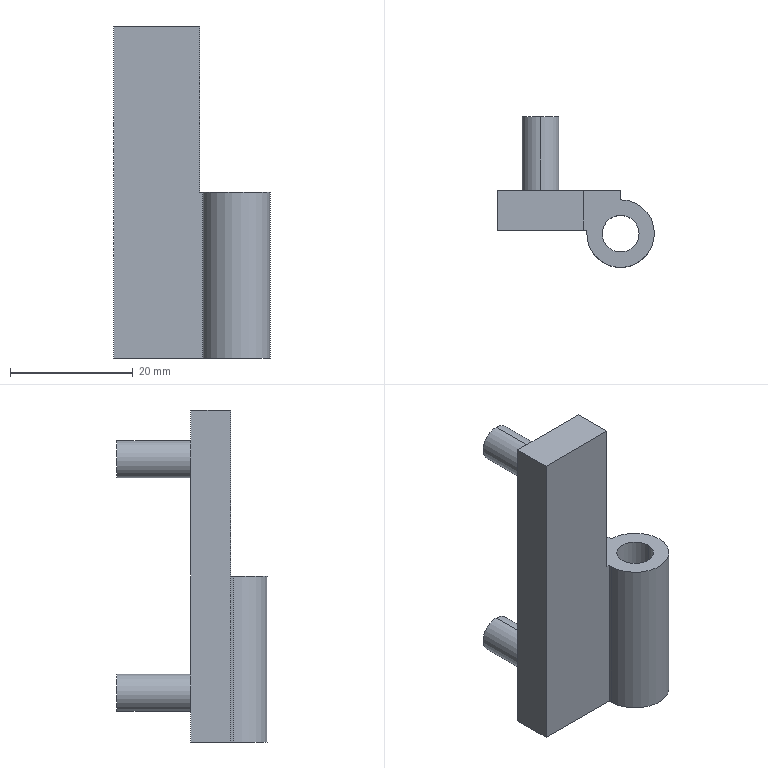Part | STEP file | Hinge leaf | 1 solid | 19 faces | box 25.5 x 24.5 x 54 mm | volume 7881 mm3 | plane 10 | cylinder 9 | commonest cylinder face diameters 6 x6 11 x3
STEP:
#1=CARTESIAN_POINT('',(0.,0.,0.));
#2=DIRECTION('',(0.,0.,1.));
#3=DIRECTION('',(1.,0.,0.));
#4=AXIS2_PLACEMENT_3D('',#1,#2,#3);
#5=CARTESIAN_POINT('',(7.,12.,43.));
#6=VERTEX_POINT('',#5);
#7=CARTESIAN_POINT('',(7.,12.,49.));
#8=VERTEX_POINT('',#7);
#9=CARTESIAN_POINT('',(7.,12.,46.));
#10=DIRECTION('',(0.,-1.,0.));
#11=DIRECTION('',(0.,0.,-1.));
#12=AXIS2_PLACEMENT_3D('',#9,#10,#11);
#13=CIRCLE('',#12,3.);
#14=CARTESIAN_POINT('',(7.,12.,46.));
#15=DIRECTION('',(0.,-1.,0.));
#16=DIRECTION('',(0.,0.,-1.));
#17=AXIS2_PLACEMENT_3D('',#14,#15,#16);
#18=CYLINDRICAL_SURFACE('',#17,3.);
#19=CARTESIAN_POINT('',(0.,0.));
#20=DIRECTION('',(1.,0.));
#21=VECTOR('',#20,1.);
#22=LINE('',#19,#21);
#23=(GEOMETRIC_REPRESENTATION_CONTEXT(2)PARAMETRIC_REPRESENTATION_CONTEXT()REPRESENTATION_CONTEXT('',''));
#24=DEFINITIONAL_REPRESENTATION('',(#22),#23);
#25=PCURVE('',#18,#24);
#26=CARTESIAN_POINT('',(7.,12.,46.));
#27=DIRECTION('',(0.,1.,0.));
#28=DIRECTION('',(0.,0.,1.));
#29=AXIS2_PLACEMENT_3D('',#26,#27,#28);
#30=PLANE('',#29);
#31=CARTESIAN_POINT('',(-3.,0.));
#32=CARTESIAN_POINT('',(-3.,5.196));
#33=CARTESIAN_POINT('',(1.5,2.598));
#34=CARTESIAN_POINT('',(6.,0.));
#35=CARTESIAN_POINT('',(1.5,-2.598));
#36=CARTESIAN_POINT('',(-3.,-5.196));
#37=CARTESIAN_POINT('',(-3.,0.));
#38=(BOUNDED_CURVE()B_SPLINE_CURVE(2,(#31,#32,#33,#34,#35,#36,#37),.UNSPECIFIED.,.T.,.F.)B_SPLINE_CURVE_WITH_KNOTS((1,2,2,2,2,1),(-2.094,0.,2.094,4.189,6.283,8.378),.UNSPECIFIED.)CURVE()GEOMETRIC_REPRESENTATION_ITEM()RATIONAL_B_SPLINE_CURVE((1.,0.5,1.,0.5,1.,0.5,1.))REPRESENTATION_ITEM(''));
#39=(GEOMETRIC_REPRESENTATION_CONTEXT(2)PARAMETRIC_REPRESENTATION_CONTEXT()REPRESENTATION_CONTEXT('',''));
#40=DEFINITIONAL_REPRESENTATION('',(#38),#39);
#41=PCURVE('',#30,#40);
#42=SURFACE_CURVE('',#13,(#25,#41),.PCURVE_S1.);
#43=EDGE_CURVE('',#6,#8,#42,.T.);
#44=ORIENTED_EDGE('',*,*,#43,.T.);
#45=CARTESIAN_POINT('',(7.,0.,49.));
#46=VERTEX_POINT('',#45);
#47=CARTESIAN_POINT('',(7.,12.,49.));
#48=DIRECTION('',(0.,-1.,0.));
#49=VECTOR('',#48,1.);
#50=LINE('',#47,#49);
#51=CARTESIAN_POINT('',(3.142,0.));
#52=DIRECTION('',(0.,1.));
#53=VECTOR('',#52,1.);
#54=LINE('',#51,#53);
#55=(GEOMETRIC_REPRESENTATION_CONTEXT(2)PARAMETRIC_REPRESENTATION_CONTEXT()REPRESENTATION_CONTEXT('',''));
#56=DEFINITIONAL_REPRESENTATION('',(#54),#55);
#57=PCURVE('',#18,#56);
#58=CARTESIAN_POINT('',(7.,12.,46.));
#59=DIRECTION('',(0.,-1.,0.));
#60=DIRECTION('',(0.,0.,-1.));
#61=AXIS2_PLACEMENT_3D('',#58,#59,#60);
#62=CYLINDRICAL_SURFACE('',#61,3.);
#63=CARTESIAN_POINT('',(3.142,0.));
#64=DIRECTION('',(0.,1.));
#65=VECTOR('',#64,1.);
#66=LINE('',#63,#65);
#67=(GEOMETRIC_REPRESENTATION_CONTEXT(2)PARAMETRIC_REPRESENTATION_CONTEXT()REPRESENTATION_CONTEXT('',''));
#68=DEFINITIONAL_REPRESENTATION('',(#66),#67);
#69=PCURVE('',#62,#68);
#70=SURFACE_CURVE('',#50,(#57,#69),.PCURVE_S1.);
#71=EDGE_CURVE('',#8,#46,#70,.T.);
#72=ORIENTED_EDGE('',*,*,#71,.T.);
#73=CARTESIAN_POINT('',(7.,0.,43.));
#74=VERTEX_POINT('',#73);
#75=CARTESIAN_POINT('',(7.,0.,46.));
#76=DIRECTION('',(0.,1.,0.));
#77=DIRECTION('',(0.,0.,-1.));
#78=AXIS2_PLACEMENT_3D('',#75,#76,#77);
#79=CIRCLE('',#78,3.);
#80=CARTESIAN_POINT('',(6.283,12.));
#81=DIRECTION('',(-1.,0.));
#82=VECTOR('',#81,1.);
#83=LINE('',#80,#82);
#84=(GEOMETRIC_REPRESENTATION_CONTEXT(2)PARAMETRIC_REPRESENTATION_CONTEXT()REPRESENTATION_CONTEXT('',''));
#85=DEFINITIONAL_REPRESENTATION('',(#83),#84);
#86=PCURVE('',#18,#85);
#87=CARTESIAN_POINT('',(0.,0.,54.));
#88=DIRECTION('',(0.,-1.,0.));
#89=DIRECTION('',(0.,0.,-1.));
#90=AXIS2_PLACEMENT_3D('',#87,#88,#89);
#91=PLANE('',#90);
#92=CARTESIAN_POINT('',(11.,7.));
#93=CARTESIAN_POINT('',(11.,1.804));
#94=CARTESIAN_POINT('',(6.5,4.402));
#95=CARTESIAN_POINT('',(2.,7.));
#96=CARTESIAN_POINT('',(6.5,9.598));
#97=CARTESIAN_POINT('',(11.,12.196));
#98=CARTESIAN_POINT('',(11.,7.));
#99=(BOUNDED_CURVE()B_SPLINE_CURVE(2,(#92,#93,#94,#95,#96,#97,#98),.UNSPECIFIED.,.T.,.F.)B_SPLINE_CURVE_WITH_KNOTS((1,2,2,2,2,1),(-2.094,0.,2.094,4.189,6.283,8.378),.UNSPECIFIED.)CURVE()GEOMETRIC_REPRESENTATION_ITEM()RATIONAL_B_SPLINE_CURVE((1.,0.5,1.,0.5,1.,0.5,1.))REPRESENTATION_ITEM(''));
#100=(GEOMETRIC_REPRESENTATION_CONTEXT(2)PARAMETRIC_REPRESENTATION_CONTEXT()REPRESENTATION_CONTEXT('',''));
#101=DEFINITIONAL_REPRESENTATION('',(#99),#100);
#102=PCURVE('',#91,#101);
#103=SURFACE_CURVE('',#79,(#86,#102),.PCURVE_S1.);
#104=EDGE_CURVE('',#46,#74,#103,.T.);
#105=ORIENTED_EDGE('',*,*,#104,.T.);
#106=CARTESIAN_POINT('',(7.,12.,43.));
#107=DIRECTION('',(0.,-1.,0.));
#108=VECTOR('',#107,1.);
#109=LINE('',#106,#108);
#110=CARTESIAN_POINT('',(0.,0.));
#111=DIRECTION('',(0.,1.));
#112=VECTOR('',#111,1.);
#113=LINE('',#110,#112);
#114=(GEOMETRIC_REPRESENTATION_CONTEXT(2)PARAMETRIC_REPRESENTATION_CONTEXT()REPRESENTATION_CONTEXT('',''));
#115=DEFINITIONAL_REPRESENTATION('',(#113),#114);
#116=PCURVE('',#18,#115);
#117=CARTESIAN_POINT('',(6.283,0.));
#118=DIRECTION('',(0.,1.));
#119=VECTOR('',#118,1.);
#120=LINE('',#117,#119);
#121=(GEOMETRIC_REPRESENTATION_CONTEXT(2)PARAMETRIC_REPRESENTATION_CONTEXT()REPRESENTATION_CONTEXT('',''));
#122=DEFINITIONAL_REPRESENTATION('',(#120),#121);
#123=PCURVE('',#62,#122);
#124=SURFACE_CURVE('',#109,(#116,#123),.PCURVE_S1.);
#125=EDGE_CURVE('',#6,#74,#124,.T.);
#126=ORIENTED_EDGE('',*,*,#125,.F.);
#127=EDGE_LOOP('',(#44,#72,#105,#126));
#128=FACE_BOUND('',#127,.T.);
#129=ADVANCED_FACE('',(#128),#18,.T.);
#130=CARTESIAN_POINT('',(7.,12.,5.));
#131=VERTEX_POINT('',#130);
#132=CARTESIAN_POINT('',(7.,12.,11.));
#133=VERTEX_POINT('',#132);
#134=CARTESIAN_POINT('',(7.,12.,8.));
#135=DIRECTION('',(0.,-1.,0.));
#136=DIRECTION('',(0.,0.,-1.));
#137=AXIS2_PLACEMENT_3D('',#134,#135,#136);
#138=CIRCLE('',#137,3.);
#139=CARTESIAN_POINT('',(7.,12.,8.));
#140=DIRECTION('',(0.,-1.,0.));
#141=DIRECTION('',(0.,0.,-1.));
#142=AXIS2_PLACEMENT_3D('',#139,#140,#141);
#143=CYLINDRICAL_SURFACE('',#142,3.);
#144=CARTESIAN_POINT('',(0.,0.));
#145=DIRECTION('',(1.,0.));
#146=VECTOR('',#145,1.);
#147=LINE('',#144,#146);
#148=(GEOMETRIC_REPRESENTATION_CONTEXT(2)PARAMETRIC_REPRESENTATION_CONTEXT()REPRESENTATION_CONTEXT('',''));
#149=DEFINITIONAL_REPRESENTATION('',(#147),#148);
#150=PCURVE('',#143,#149);
#151=CARTESIAN_POINT('',(7.,12.,8.));
#152=DIRECTION('',(0.,1.,0.));
#153=DIRECTION('',(0.,0.,1.));
#154=AXIS2_PLACEMENT_3D('',#151,#152,#153);
#155=PLANE('',#154);
#156=CARTESIAN_POINT('',(-3.,0.));
#157=CARTESIAN_POINT('',(-3.,5.196));
#158=CARTESIAN_POINT('',(1.5,2.598));
#159=CARTESIAN_POINT('',(6.,0.));
#160=CARTESIAN_POINT('',(1.5,-2.598));
#161=CARTESIAN_POINT('',(-3.,-5.196));
#162=CARTESIAN_POINT('',(-3.,0.));
#163=(BOUNDED_CURVE()B_SPLINE_CURVE(2,(#156,#157,#158,#159,#160,#161,#162),.UNSPECIFIED.,.T.,.F.)B_SPLINE_CURVE_WITH_KNOTS((1,2,2,2,2,1),(-2.094,0.,2.094,4.189,6.283,8.378),.UNSPECIFIED.)CURVE()GEOMETRIC_REPRESENTATION_ITEM()RATIONAL_B_SPLINE_CURVE((1.,0.5,1.,0.5,1.,0.5,1.))REPRESENTATION_ITEM(''));
#164=(GEOMETRIC_REPRESENTATION_CONTEXT(2)PARAMETRIC_REPRESENTATION_CONTEXT()REPRESENTATION_CONTEXT('',''));
#165=DEFINITIONAL_REPRESENTATION('',(#163),#164);
#166=PCURVE('',#155,#165);
#167=SURFACE_CURVE('',#138,(#150,#166),.PCURVE_S1.);
#168=EDGE_CURVE('',#131,#133,#167,.T.);
#169=ORIENTED_EDGE('',*,*,#168,.T.);
#170=CARTESIAN_POINT('',(7.,0.,11.));
#171=VERTEX_POINT('',#170);
#172=CARTESIAN_POINT('',(7.,12.,11.));
#173=DIRECTION('',(0.,-1.,0.));
#174=VECTOR('',#173,1.);
#175=LINE('',#172,#174);
#176=CARTESIAN_POINT('',(3.142,0.));
#177=DIRECTION('',(0.,1.));
#178=VECTOR('',#177,1.);
#179=LINE('',#176,#178);
#180=(GEOMETRIC_REPRESENTATION_CONTEXT(2)PARAMETRIC_REPRESENTATION_CONTEXT()REPRESENTATION_CONTEXT('',''));
#181=DEFINITIONAL_REPRESENTATION('',(#179),#180);
#182=PCURVE('',#143,#181);
#183=CARTESIAN_POINT('',(7.,12.,8.));
#184=DIRECTION('',(0.,-1.,0.));
#185=DIRECTION('',(0.,0.,-1.));
#186=AXIS2_PLACEMENT_3D('',#183,#184,#185);
#187=CYLINDRICAL_SURFACE('',#186,3.);
#188=CARTESIAN_POINT('',(3.142,0.));
#189=DIRECTION('',(0.,1.));
#190=VECTOR('',#189,1.);
#191=LINE('',#188,#190);
#192=(GEOMETRIC_REPRESENTATION_CONTEXT(2)PARAMETRIC_REPRESENTATION_CONTEXT()REPRESENTATION_CONTEXT('',''));
#193=DEFINITIONAL_REPRESENTATION('',(#191),#192);
#194=PCURVE('',#187,#193);
#195=SURFACE_CURVE('',#175,(#182,#194),.PCURVE_S1.);
#196=EDGE_CURVE('',#133,#171,#195,.T.);
#197=ORIENTED_EDGE('',*,*,#196,.T.);
#198=CARTESIAN_POINT('',(7.,0.,5.));
#199=VERTEX_POINT('',#198);
#200=CARTESIAN_POINT('',(7.,0.,8.));
#201=DIRECTION('',(0.,1.,0.));
#202=DIRECTION('',(0.,0.,-1.));
#203=AXIS2_PLACEMENT_3D('',#200,#201,#202);
#204=CIRCLE('',#203,3.);
#205=CARTESIAN_POINT('',(6.283,12.));
#206=DIRECTION('',(-1.,0.));
#207=VECTOR('',#206,1.);
#208=LINE('',#205,#207);
#209=(GEOMETRIC_REPRESENTATION_CONTEXT(2)PARAMETRIC_REPRESENTATION_CONTEXT()REPRESENTATION_CONTEXT('',''));
#210=DEFINITIONAL_REPRESENTATION('',(#208),#209);
#211=PCURVE('',#143,#210);
#212=CARTESIAN_POINT('',(49.,7.));
#213=CARTESIAN_POINT('',(49.,1.804));
#214=CARTESIAN_POINT('',(44.5,4.402));
#215=CARTESIAN_POINT('',(40.,7.));
#216=CARTESIAN_POINT('',(44.5,9.598));
#217=CARTESIAN_POINT('',(49.,12.196));
#218=CARTESIAN_POINT('',(49.,7.));
#219=(BOUNDED_CURVE()B_SPLINE_CURVE(2,(#212,#213,#214,#215,#216,#217,#218),.UNSPECIFIED.,.T.,.F.)B_SPLINE_CURVE_WITH_KNOTS((1,2,2,2,2,1),(-2.094,0.,2.094,4.189,6.283,8.378),.UNSPECIFIED.)CURVE()GEOMETRIC_REPRESENTATION_ITEM()RATIONAL_B_SPLINE_CURVE((1.,0.5,1.,0.5,1.,0.5,1.))REPRESENTATION_ITEM(''));
#220=(GEOMETRIC_REPRESENTATION_CONTEXT(2)PARAMETRIC_REPRESENTATION_CONTEXT()REPRESENTATION_CONTEXT('',''));
#221=DEFINITIONAL_REPRESENTATION('',(#219),#220);
#222=PCURVE('',#91,#221);
#223=SURFACE_CURVE('',#204,(#211,#222),.PCURVE_S1.);
#224=EDGE_CURVE('',#171,#199,#223,.T.);
#225=ORIENTED_EDGE('',*,*,#224,.T.);
#226=CARTESIAN_POINT('',(7.,12.,5.));
#227=DIRECTION('',(0.,-1.,0.));
#228=VECTOR('',#227,1.);
#229=LINE('',#226,#228);
#230=CARTESIAN_POINT('',(0.,0.));
#231=DIRECTION('',(0.,1.));
#232=VECTOR('',#231,1.);
#233=LINE('',#230,#232);
#234=(GEOMETRIC_REPRESENTATION_CONTEXT(2)PARAMETRIC_REPRESENTATION_CONTEXT()REPRESENTATION_CONTEXT('',''));
#235=DEFINITIONAL_REPRESENTATION('',(#233),#234);
#236=PCURVE('',#143,#235);
#237=CARTESIAN_POINT('',(6.283,0.));
#238=DIRECTION('',(0.,1.));
#239=VECTOR('',#238,1.);
#240=LINE('',#237,#239);
#241=(GEOMETRIC_REPRESENTATION_CONTEXT(2)PARAMETRIC_REPRESENTATION_CONTEXT()REPRESENTATION_CONTEXT('',''));
#242=DEFINITIONAL_REPRESENTATION('',(#240),#241);
#243=PCURVE('',#187,#242);
#244=SURFACE_CURVE('',#229,(#236,#243),.PCURVE_S1.);
#245=EDGE_CURVE('',#131,#199,#244,.T.);
#246=ORIENTED_EDGE('',*,*,#245,.F.);
#247=EDGE_LOOP('',(#169,#197,#225,#246));
#248=FACE_BOUND('',#247,.T.);
#249=ADVANCED_FACE('',(#248),#143,.T.);
#250=CARTESIAN_POINT('',(25.5,-7.,27.));
#251=VERTEX_POINT('',#250);
#252=CARTESIAN_POINT('',(20.,-1.5,27.));
#253=VERTEX_POINT('',#252);
#254=CARTESIAN_POINT('',(20.,-7.,27.));
#255=DIRECTION('',(0.,0.,1.));
#256=DIRECTION('',(-1.,0.,0.));
#257=AXIS2_PLACEMENT_3D('',#254,#255,#256);
#258=CIRCLE('',#257,5.5);
#259=CARTESIAN_POINT('',(20.,-7.,54.));
#260=DIRECTION('',(0.,0.,-1.));
#261=DIRECTION('',(-1.,0.,0.));
#262=AXIS2_PLACEMENT_3D('',#259,#260,#261);
#263=CYLINDRICAL_SURFACE('',#262,5.5);
#264=CARTESIAN_POINT('',(6.283,27.));
#265=DIRECTION('',(-1.,0.));
#266=VECTOR('',#265,1.);
#267=LINE('',#264,#266);
#268=(GEOMETRIC_REPRESENTATION_CONTEXT(2)PARAMETRIC_REPRESENTATION_CONTEXT()REPRESENTATION_CONTEXT('',''));
#269=DEFINITIONAL_REPRESENTATION('',(#267),#268);
#270=PCURVE('',#263,#269);
#271=CARTESIAN_POINT('',(14.,-14.282,27.));
#272=DIRECTION('',(0.,0.,1.));
#273=DIRECTION('',(1.,0.,0.));
#274=AXIS2_PLACEMENT_3D('',#271,#272,#273);
#275=PLANE('',#274);
#276=CARTESIAN_POINT('',(6.,7.282));
#277=DIRECTION('',(-1.,0.));
#278=AXIS2_PLACEMENT_2D('',#276,#277);
#279=CIRCLE('',#278,5.5);
#280=(GEOMETRIC_REPRESENTATION_CONTEXT(2)PARAMETRIC_REPRESENTATION_CONTEXT()REPRESENTATION_CONTEXT('',''));
#281=DEFINITIONAL_REPRESENTATION('',(#279),#280);
#282=PCURVE('',#275,#281);
#283=SURFACE_CURVE('',#258,(#270,#282),.PCURVE_S1.);
#284=EDGE_CURVE('',#251,#253,#283,.T.);
#285=ORIENTED_EDGE('',*,*,#284,.F.);
#286=CARTESIAN_POINT('',(25.5,-7.,0.));
#287=VERTEX_POINT('',#286);
#288=CARTESIAN_POINT('',(25.5,-7.,54.));
#289=DIRECTION('',(0.,0.,-1.));
#290=VECTOR('',#289,1.);
#291=LINE('',#288,#290);
#292=CARTESIAN_POINT('',(3.142,0.));
#293=DIRECTION('',(0.,1.));
#294=VECTOR('',#293,1.);
#295=LINE('',#292,#294);
#296=(GEOMETRIC_REPRESENTATION_CONTEXT(2)PARAMETRIC_REPRESENTATION_CONTEXT()REPRESENTATION_CONTEXT('',''));
#297=DEFINITIONAL_REPRESENTATION('',(#295),#296);
#298=PCURVE('',#263,#297);
#299=CARTESIAN_POINT('',(20.,-7.,54.));
#300=DIRECTION('',(0.,0.,-1.));
#301=DIRECTION('',(-1.,0.,0.));
#302=AXIS2_PLACEMENT_3D('',#299,#300,#301);
#303=CYLINDRICAL_SURFACE('',#302,5.5);
#304=CARTESIAN_POINT('',(3.142,0.));
#305=DIRECTION('',(0.,1.));
#306=VECTOR('',#305,1.);
#307=LINE('',#304,#306);
#308=(GEOMETRIC_REPRESENTATION_CONTEXT(2)PARAMETRIC_REPRESENTATION_CONTEXT()REPRESENTATION_CONTEXT('',''));
#309=DEFINITIONAL_REPRESENTATION('',(#307),#308);
#310=PCURVE('',#303,#309);
#311=SURFACE_CURVE('',#291,(#298,#310),.PCURVE_S1.);
#312=EDGE_CURVE('',#251,#287,#311,.T.);
#313=ORIENTED_EDGE('',*,*,#312,.T.);
#314=CARTESIAN_POINT('',(20.,-1.5,0.));
#315=VERTEX_POINT('',#314);
#316=CARTESIAN_POINT('',(20.,-7.,0.));
#317=DIRECTION('',(0.,0.,1.));
#318=DIRECTION('',(-1.,0.,0.));
#319=AXIS2_PLACEMENT_3D('',#316,#317,#318);
#320=CIRCLE('',#319,5.5);
#321=CARTESIAN_POINT('',(6.283,54.));
#322=DIRECTION('',(-1.,0.));
#323=VECTOR('',#322,1.);
#324=LINE('',#321,#323);
#325=(GEOMETRIC_REPRESENTATION_CONTEXT(2)PARAMETRIC_REPRESENTATION_CONTEXT()REPRESENTATION_CONTEXT('',''));
#326=DEFINITIONAL_REPRESENTATION('',(#324),#325);
#327=PCURVE('',#263,#326);
#328=CARTESIAN_POINT('',(20.,-7.,0.));
#329=DIRECTION('',(0.,0.,1.));
#330=DIRECTION('',(1.,0.,0.));
#331=AXIS2_PLACEMENT_3D('',#328,#329,#330);
#332=PLANE('',#331);
#333=CARTESIAN_POINT('',(0.,0.));
#334=DIRECTION('',(-1.,0.));
#335=AXIS2_PLACEMENT_2D('',#333,#334);
#336=CIRCLE('',#335,5.5);
#337=(GEOMETRIC_REPRESENTATION_CONTEXT(2)PARAMETRIC_REPRESENTATION_CONTEXT()REPRESENTATION_CONTEXT('',''));
#338=DEFINITIONAL_REPRESENTATION('',(#336),#337);
#339=PCURVE('',#332,#338);
#340=SURFACE_CURVE('',#320,(#327,#339),.PCURVE_S1.);
#341=EDGE_CURVE('',#287,#315,#340,.T.);
#342=ORIENTED_EDGE('',*,*,#341,.T.);
#343=CARTESIAN_POINT('',(20.,-1.5,54.));
#344=DIRECTION('',(0.,0.,1.));
#345=VECTOR('',#344,1.);
#346=LINE('',#343,#345);
#347=CARTESIAN_POINT('',(1.571,0.));
#348=DIRECTION('',(0.,-1.));
#349=VECTOR('',#348,1.);
#350=LINE('',#347,#349);
#351=(GEOMETRIC_REPRESENTATION_CONTEXT(2)PARAMETRIC_REPRESENTATION_CONTEXT()REPRESENTATION_CONTEXT('',''));
#352=DEFINITIONAL_REPRESENTATION('',(#350),#351);
#353=PCURVE('',#263,#352);
#354=CARTESIAN_POINT('',(20.,0.,54.));
#355=DIRECTION('',(-1.,0.,0.));
#356=DIRECTION('',(0.,0.,1.));
#357=AXIS2_PLACEMENT_3D('',#354,#355,#356);
#358=PLANE('',#357);
#359=CARTESIAN_POINT('',(0.,-1.5));
#360=DIRECTION('',(1.,0.));
#361=VECTOR('',#360,1.);
#362=LINE('',#359,#361);
#363=(GEOMETRIC_REPRESENTATION_CONTEXT(2)PARAMETRIC_REPRESENTATION_CONTEXT()REPRESENTATION_CONTEXT('',''));
#364=DEFINITIONAL_REPRESENTATION('',(#362),#363);
#365=PCURVE('',#358,#364);
#366=SURFACE_CURVE('',#346,(#353,#365),.PCURVE_S1.);
#367=EDGE_CURVE('',#315,#253,#366,.T.);
#368=ORIENTED_EDGE('',*,*,#367,.T.);
#369=EDGE_LOOP('',(#285,#313,#342,#368));
#370=FACE_BOUND('',#369,.T.);
#371=ADVANCED_FACE('',(#370),#263,.T.);
#372=ORIENTED_EDGE('',*,*,#312,.F.);
#373=CARTESIAN_POINT('',(14.5,-7.,27.));
#374=VERTEX_POINT('',#373);
#375=CARTESIAN_POINT('',(20.,-7.,27.));
#376=DIRECTION('',(0.,0.,1.));
#377=DIRECTION('',(-1.,0.,0.));
#378=AXIS2_PLACEMENT_3D('',#375,#376,#377);
#379=CIRCLE('',#378,5.5);
#380=CARTESIAN_POINT('',(6.283,27.));
#381=DIRECTION('',(-1.,0.));
#382=VECTOR('',#381,1.);
#383=LINE('',#380,#382);
#384=(GEOMETRIC_REPRESENTATION_CONTEXT(2)PARAMETRIC_REPRESENTATION_CONTEXT()REPRESENTATION_CONTEXT('',''));
#385=DEFINITIONAL_REPRESENTATION('',(#383),#384);
#386=PCURVE('',#303,#385);
#387=CARTESIAN_POINT('',(6.,7.282));
#388=DIRECTION('',(-1.,0.));
#389=AXIS2_PLACEMENT_2D('',#387,#388);
#390=CIRCLE('',#389,5.5);
#391=(GEOMETRIC_REPRESENTATION_CONTEXT(2)PARAMETRIC_REPRESENTATION_CONTEXT()REPRESENTATION_CONTEXT('',''));
#392=DEFINITIONAL_REPRESENTATION('',(#390),#391);
#393=PCURVE('',#275,#392);
#394=SURFACE_CURVE('',#379,(#386,#393),.PCURVE_S1.);
#395=EDGE_CURVE('',#374,#251,#394,.T.);
#396=ORIENTED_EDGE('',*,*,#395,.F.);
#397=CARTESIAN_POINT('',(14.5,-7.,0.));
#398=VERTEX_POINT('',#397);
#399=CARTESIAN_POINT('',(14.5,-7.,54.));
#400=DIRECTION('',(0.,0.,-1.));
#401=VECTOR('',#400,1.);
#402=LINE('',#399,#401);
#403=CARTESIAN_POINT('',(6.283,0.));
#404=DIRECTION('',(0.,1.));
#405=VECTOR('',#404,1.);
#406=LINE('',#403,#405);
#407=(GEOMETRIC_REPRESENTATION_CONTEXT(2)PARAMETRIC_REPRESENTATION_CONTEXT()REPRESENTATION_CONTEXT('',''));
#408=DEFINITIONAL_REPRESENTATION('',(#406),#407);
#409=PCURVE('',#303,#408);
#410=CARTESIAN_POINT('',(20.,-7.,54.));
#411=DIRECTION('',(0.,0.,-1.));
#412=DIRECTION('',(-1.,0.,0.));
#413=AXIS2_PLACEMENT_3D('',#410,#411,#412);
#414=CYLINDRICAL_SURFACE('',#413,5.5);
#415=CARTESIAN_POINT('',(0.,0.));
#416=DIRECTION('',(0.,1.));
#417=VECTOR('',#416,1.);
#418=LINE('',#415,#417);
#419=(GEOMETRIC_REPRESENTATION_CONTEXT(2)PARAMETRIC_REPRESENTATION_CONTEXT()REPRESENTATION_CONTEXT('',''));
#420=DEFINITIONAL_REPRESENTATION('',(#418),#419);
#421=PCURVE('',#414,#420);
#422=SURFACE_CURVE('',#402,(#409,#421),.PCURVE_S1.);
#423=EDGE_CURVE('',#374,#398,#422,.T.);
#424=ORIENTED_EDGE('',*,*,#423,.T.);
#425=CARTESIAN_POINT('',(20.,-7.,0.));
#426=DIRECTION('',(0.,0.,1.));
#427=DIRECTION('',(-1.,0.,0.));
#428=AXIS2_PLACEMENT_3D('',#425,#426,#427);
#429=CIRCLE('',#428,5.5);
#430=CARTESIAN_POINT('',(6.283,54.));
#431=DIRECTION('',(-1.,0.));
#432=VECTOR('',#431,1.);
#433=LINE('',#430,#432);
#434=(GEOMETRIC_REPRESENTATION_CONTEXT(2)PARAMETRIC_REPRESENTATION_CONTEXT()REPRESENTATION_CONTEXT('',''));
#435=DEFINITIONAL_REPRESENTATION('',(#433),#434);
#436=PCURVE('',#303,#435);
#437=CARTESIAN_POINT('',(0.,0.));
#438=DIRECTION('',(-1.,0.));
#439=AXIS2_PLACEMENT_2D('',#437,#438);
#440=CIRCLE('',#439,5.5);
#441=(GEOMETRIC_REPRESENTATION_CONTEXT(2)PARAMETRIC_REPRESENTATION_CONTEXT()REPRESENTATION_CONTEXT('',''));
#442=DEFINITIONAL_REPRESENTATION('',(#440),#441);
#443=PCURVE('',#332,#442);
#444=SURFACE_CURVE('',#429,(#436,#443),.PCURVE_S1.);
#445=EDGE_CURVE('',#398,#287,#444,.T.);
#446=ORIENTED_EDGE('',*,*,#445,.T.);
#447=EDGE_LOOP('',(#372,#396,#424,#446));
#448=FACE_BOUND('',#447,.T.);
#449=ADVANCED_FACE('',(#448),#303,.T.);
#450=CARTESIAN_POINT('',(17.,-7.,27.));
#451=VERTEX_POINT('',#450);
#452=CARTESIAN_POINT('',(17.,-7.,0.));
#453=VERTEX_POINT('',#452);
#454=CARTESIAN_POINT('',(17.,-7.,54.));
#455=DIRECTION('',(0.,0.,-1.));
#456=VECTOR('',#455,1.);
#457=LINE('',#454,#456);
#458=CARTESIAN_POINT('',(20.,-7.,54.));
#459=DIRECTION('',(0.,0.,-1.));
#460=DIRECTION('',(-1.,0.,0.));
#461=AXIS2_PLACEMENT_3D('',#458,#459,#460);
#462=CYLINDRICAL_SURFACE('',#461,3.);
#463=CARTESIAN_POINT('',(6.283,0.));
#464=DIRECTION('',(0.,1.));
#465=VECTOR('',#464,1.);
#466=LINE('',#463,#465);
#467=(GEOMETRIC_REPRESENTATION_CONTEXT(2)PARAMETRIC_REPRESENTATION_CONTEXT()REPRESENTATION_CONTEXT('',''));
#468=DEFINITIONAL_REPRESENTATION('',(#466),#467);
#469=PCURVE('',#462,#468);
#470=CARTESIAN_POINT('',(20.,-7.,54.));
#471=DIRECTION('',(0.,0.,-1.));
#472=DIRECTION('',(-1.,0.,0.));
#473=AXIS2_PLACEMENT_3D('',#470,#471,#472);
#474=CYLINDRICAL_SURFACE('',#473,3.);
#475=CARTESIAN_POINT('',(0.,0.));
#476=DIRECTION('',(0.,1.));
#477=VECTOR('',#476,1.);
#478=LINE('',#475,#477);
#479=(GEOMETRIC_REPRESENTATION_CONTEXT(2)PARAMETRIC_REPRESENTATION_CONTEXT()REPRESENTATION_CONTEXT('',''));
#480=DEFINITIONAL_REPRESENTATION('',(#478),#479);
#481=PCURVE('',#474,#480);
#482=SURFACE_CURVE('',#457,(#469,#481),.PCURVE_S1.);
#483=EDGE_CURVE('',#451,#453,#482,.T.);
#484=ORIENTED_EDGE('',*,*,#483,.T.);
#485=CARTESIAN_POINT('',(23.,-7.,0.));
#486=VERTEX_POINT('',#485);
#487=CARTESIAN_POINT('',(20.,-7.,0.));
#488=DIRECTION('',(0.,0.,-1.));
#489=DIRECTION('',(-1.,0.,0.));
#490=AXIS2_PLACEMENT_3D('',#487,#488,#489);
#491=CIRCLE('',#490,3.);
#492=CARTESIAN_POINT('',(0.,54.));
#493=DIRECTION('',(1.,0.));
#494=VECTOR('',#493,1.);
#495=LINE('',#492,#494);
#496=(GEOMETRIC_REPRESENTATION_CONTEXT(2)PARAMETRIC_REPRESENTATION_CONTEXT()REPRESENTATION_CONTEXT('',''));
#497=DEFINITIONAL_REPRESENTATION('',(#495),#496);
#498=PCURVE('',#462,#497);
#499=CARTESIAN_POINT('',(-3.,0.));
#500=CARTESIAN_POINT('',(-3.,5.196));
#501=CARTESIAN_POINT('',(1.5,2.598));
#502=CARTESIAN_POINT('',(6.,0.));
#503=CARTESIAN_POINT('',(1.5,-2.598));
#504=CARTESIAN_POINT('',(-3.,-5.196));
#505=CARTESIAN_POINT('',(-3.,0.));
#506=(BOUNDED_CURVE()B_SPLINE_CURVE(2,(#499,#500,#501,#502,#503,#504,#505),.UNSPECIFIED.,.T.,.F.)B_SPLINE_CURVE_WITH_KNOTS((1,2,2,2,2,1),(-2.094,0.,2.094,4.189,6.283,8.378),.UNSPECIFIED.)CURVE()GEOMETRIC_REPRESENTATION_ITEM()RATIONAL_B_SPLINE_CURVE((1.,0.5,1.,0.5,1.,0.5,1.))REPRESENTATION_ITEM(''));
#507=(GEOMETRIC_REPRESENTATION_CONTEXT(2)PARAMETRIC_REPRESENTATION_CONTEXT()REPRESENTATION_CONTEXT('',''));
#508=DEFINITIONAL_REPRESENTATION('',(#506),#507);
#509=PCURVE('',#332,#508);
#510=SURFACE_CURVE('',#491,(#498,#509),.PCURVE_S1.);
#511=EDGE_CURVE('',#486,#453,#510,.T.);
#512=ORIENTED_EDGE('',*,*,#511,.F.);
#513=CARTESIAN_POINT('',(23.,-7.,27.));
#514=VERTEX_POINT('',#513);
#515=CARTESIAN_POINT('',(23.,-7.,54.));
#516=DIRECTION('',(0.,0.,-1.));
#517=VECTOR('',#516,1.);
#518=LINE('',#515,#517);
#519=CARTESIAN_POINT('',(3.142,0.));
#520=DIRECTION('',(0.,1.));
#521=VECTOR('',#520,1.);
#522=LINE('',#519,#521);
#523=(GEOMETRIC_REPRESENTATION_CONTEXT(2)PARAMETRIC_REPRESENTATION_CONTEXT()REPRESENTATION_CONTEXT('',''));
#524=DEFINITIONAL_REPRESENTATION('',(#522),#523);
#525=PCURVE('',#462,#524);
#526=CARTESIAN_POINT('',(3.142,0.));
#527=DIRECTION('',(0.,1.));
#528=VECTOR('',#527,1.);
#529=LINE('',#526,#528);
#530=(GEOMETRIC_REPRESENTATION_CONTEXT(2)PARAMETRIC_REPRESENTATION_CONTEXT()REPRESENTATION_CONTEXT('',''));
#531=DEFINITIONAL_REPRESENTATION('',(#529),#530);
#532=PCURVE('',#474,#531);
#533=SURFACE_CURVE('',#518,(#525,#532),.PCURVE_S1.);
#534=EDGE_CURVE('',#514,#486,#533,.T.);
#535=ORIENTED_EDGE('',*,*,#534,.F.);
#536=CARTESIAN_POINT('',(20.,-7.,27.));
#537=DIRECTION('',(0.,0.,-1.));
#538=DIRECTION('',(-1.,0.,0.));
#539=AXIS2_PLACEMENT_3D('',#536,#537,#538);
#540=CIRCLE('',#539,3.);
#541=CARTESIAN_POINT('',(0.,27.));
#542=DIRECTION('',(1.,0.));
#543=VECTOR('',#542,1.);
#544=LINE('',#541,#543);
#545=(GEOMETRIC_REPRESENTATION_CONTEXT(2)PARAMETRIC_REPRESENTATION_CONTEXT()REPRESENTATION_CONTEXT('',''));
#546=DEFINITIONAL_REPRESENTATION('',(#544),#545);
#547=PCURVE('',#462,#546);
#548=CARTESIAN_POINT('',(3.,7.282));
#549=CARTESIAN_POINT('',(3.,12.478));
#550=CARTESIAN_POINT('',(7.5,9.88));
#551=CARTESIAN_POINT('',(12.,7.282));
#552=CARTESIAN_POINT('',(7.5,4.684));
#553=CARTESIAN_POINT('',(3.,2.085));
#554=CARTESIAN_POINT('',(3.,7.282));
#555=(BOUNDED_CURVE()B_SPLINE_CURVE(2,(#548,#549,#550,#551,#552,#553,#554),.UNSPECIFIED.,.T.,.F.)B_SPLINE_CURVE_WITH_KNOTS((1,2,2,2,2,1),(-2.094,0.,2.094,4.189,6.283,8.378),.UNSPECIFIED.)CURVE()GEOMETRIC_REPRESENTATION_ITEM()RATIONAL_B_SPLINE_CURVE((1.,0.5,1.,0.5,1.,0.5,1.))REPRESENTATION_ITEM(''));
#556=(GEOMETRIC_REPRESENTATION_CONTEXT(2)PARAMETRIC_REPRESENTATION_CONTEXT()REPRESENTATION_CONTEXT('',''));
#557=DEFINITIONAL_REPRESENTATION('',(#555),#556);
#558=PCURVE('',#275,#557);
#559=SURFACE_CURVE('',#540,(#547,#558),.PCURVE_S1.);
#560=EDGE_CURVE('',#514,#451,#559,.T.);
#561=ORIENTED_EDGE('',*,*,#560,.T.);
#562=EDGE_LOOP('',(#484,#512,#535,#561));
#563=FACE_BOUND('',#562,.F.);
#564=ADVANCED_FACE('',(#563),#462,.F.);
#565=CARTESIAN_POINT('',(7.,0.,46.));
#566=DIRECTION('',(0.,1.,0.));
#567=DIRECTION('',(0.,0.,-1.));
#568=AXIS2_PLACEMENT_3D('',#565,#566,#567);
#569=CIRCLE('',#568,3.);
#570=CARTESIAN_POINT('',(11.,7.));
#571=CARTESIAN_POINT('',(11.,1.804));
#572=CARTESIAN_POINT('',(6.5,4.402));
#573=CARTESIAN_POINT('',(2.,7.));
#574=CARTESIAN_POINT('',(6.5,9.598));
#575=CARTESIAN_POINT('',(11.,12.196));
#576=CARTESIAN_POINT('',(11.,7.));
#577=(BOUNDED_CURVE()B_SPLINE_CURVE(2,(#570,#571,#572,#573,#574,#575,#576),.UNSPECIFIED.,.T.,.F.)B_SPLINE_CURVE_WITH_KNOTS((1,2,2,2,2,1),(-2.094,0.,2.094,4.189,6.283,8.378),.UNSPECIFIED.)CURVE()GEOMETRIC_REPRESENTATION_ITEM()RATIONAL_B_SPLINE_CURVE((1.,0.5,1.,0.5,1.,0.5,1.))REPRESENTATION_ITEM(''));
#578=(GEOMETRIC_REPRESENTATION_CONTEXT(2)PARAMETRIC_REPRESENTATION_CONTEXT()REPRESENTATION_CONTEXT('',''));
#579=DEFINITIONAL_REPRESENTATION('',(#577),#578);
#580=PCURVE('',#91,#579);
#581=CARTESIAN_POINT('',(6.283,12.));
#582=DIRECTION('',(-1.,0.));
#583=VECTOR('',#582,1.);
#584=LINE('',#581,#583);
#585=(GEOMETRIC_REPRESENTATION_CONTEXT(2)PARAMETRIC_REPRESENTATION_CONTEXT()REPRESENTATION_CONTEXT('',''));
#586=DEFINITIONAL_REPRESENTATION('',(#584),#585);
#587=PCURVE('',#62,#586);
#588=SURFACE_CURVE('',#569,(#580,#587),.PCURVE_S1.);
#589=EDGE_CURVE('',#74,#46,#588,.T.);
#590=ORIENTED_EDGE('',*,*,#589,.F.);
#591=ORIENTED_EDGE('',*,*,#104,.F.);
#592=EDGE_LOOP('',(#590,#591));
#593=FACE_BOUND('',#592,.T.);
#594=CARTESIAN_POINT('',(14.,0.,27.));
#595=VERTEX_POINT('',#594);
#596=CARTESIAN_POINT('',(14.,0.,54.));
#597=VERTEX_POINT('',#596);
#598=CARTESIAN_POINT('',(14.,0.,54.));
#599=DIRECTION('',(0.,0.,1.));
#600=VECTOR('',#599,1.);
#601=LINE('',#598,#600);
#602=CARTESIAN_POINT('',(0.,14.));
#603=DIRECTION('',(-1.,0.));
#604=VECTOR('',#603,1.);
#605=LINE('',#602,#604);
#606=(GEOMETRIC_REPRESENTATION_CONTEXT(2)PARAMETRIC_REPRESENTATION_CONTEXT()REPRESENTATION_CONTEXT('',''));
#607=DEFINITIONAL_REPRESENTATION('',(#605),#606);
#608=PCURVE('',#91,#607);
#609=CARTESIAN_POINT('',(14.,2.063,27.));
#610=DIRECTION('',(-1.,0.,0.));
#611=DIRECTION('',(0.,-1.,0.));
#612=AXIS2_PLACEMENT_3D('',#609,#610,#611);
#613=PLANE('',#612);
#614=CARTESIAN_POINT('',(2.063,27.));
#615=DIRECTION('',(0.,1.));
#616=VECTOR('',#615,1.);
#617=LINE('',#614,#616);
#618=(GEOMETRIC_REPRESENTATION_CONTEXT(2)PARAMETRIC_REPRESENTATION_CONTEXT()REPRESENTATION_CONTEXT('',''));
#619=DEFINITIONAL_REPRESENTATION('',(#617),#618);
#620=PCURVE('',#613,#619);
#621=SURFACE_CURVE('',#601,(#608,#620),.PCURVE_S1.);
#622=EDGE_CURVE('',#595,#597,#621,.T.);
#623=ORIENTED_EDGE('',*,*,#622,.F.);
#624=CARTESIAN_POINT('',(20.,0.,27.));
#625=VERTEX_POINT('',#624);
#626=CARTESIAN_POINT('',(0.,0.,27.));
#627=DIRECTION('',(-1.,0.,0.));
#628=VECTOR('',#627,1.);
#629=LINE('',#626,#628);
#630=CARTESIAN_POINT('',(27.,0.));
#631=DIRECTION('',(0.,-1.));
#632=VECTOR('',#631,1.);
#633=LINE('',#630,#632);
#634=(GEOMETRIC_REPRESENTATION_CONTEXT(2)PARAMETRIC_REPRESENTATION_CONTEXT()REPRESENTATION_CONTEXT('',''));
#635=DEFINITIONAL_REPRESENTATION('',(#633),#634);
#636=PCURVE('',#91,#635);
#637=CARTESIAN_POINT('',(-14.,14.282));
#638=DIRECTION('',(-1.,0.));
#639=VECTOR('',#638,1.);
#640=LINE('',#637,#639);
#641=(GEOMETRIC_REPRESENTATION_CONTEXT(2)PARAMETRIC_REPRESENTATION_CONTEXT()REPRESENTATION_CONTEXT('',''));
#642=DEFINITIONAL_REPRESENTATION('',(#640),#641);
#643=PCURVE('',#275,#642);
#644=SURFACE_CURVE('',#629,(#636,#643),.PCURVE_S1.);
#645=EDGE_CURVE('',#625,#595,#644,.T.);
#646=ORIENTED_EDGE('',*,*,#645,.F.);
#647=CARTESIAN_POINT('',(20.,0.,0.));
#648=VERTEX_POINT('',#647);
#649=CARTESIAN_POINT('',(20.,0.,54.));
#650=DIRECTION('',(0.,0.,1.));
#651=VECTOR('',#650,1.);
#652=LINE('',#649,#651);
#653=CARTESIAN_POINT('',(0.,20.));
#654=DIRECTION('',(-1.,0.));
#655=VECTOR('',#654,1.);
#656=LINE('',#653,#655);
#657=(GEOMETRIC_REPRESENTATION_CONTEXT(2)PARAMETRIC_REPRESENTATION_CONTEXT()REPRESENTATION_CONTEXT('',''));
#658=DEFINITIONAL_REPRESENTATION('',(#656),#657);
#659=PCURVE('',#91,#658);
#660=CARTESIAN_POINT('',(0.,0.));
#661=DIRECTION('',(1.,0.));
#662=VECTOR('',#661,1.);
#663=LINE('',#660,#662);
#664=(GEOMETRIC_REPRESENTATION_CONTEXT(2)PARAMETRIC_REPRESENTATION_CONTEXT()REPRESENTATION_CONTEXT('',''));
#665=DEFINITIONAL_REPRESENTATION('',(#663),#664);
#666=PCURVE('',#358,#665);
#667=SURFACE_CURVE('',#652,(#659,#666),.PCURVE_S1.);
#668=EDGE_CURVE('',#648,#625,#667,.T.);
#669=ORIENTED_EDGE('',*,*,#668,.F.);
#670=CARTESIAN_POINT('',(0.,0.,0.));
#671=VERTEX_POINT('',#670);
#672=CARTESIAN_POINT('',(0.,0.,0.));
#673=DIRECTION('',(1.,0.,0.));
#674=VECTOR('',#673,1.);
#675=LINE('',#672,#674);
#676=CARTESIAN_POINT('',(54.,0.));
#677=DIRECTION('',(0.,1.));
#678=VECTOR('',#677,1.);
#679=LINE('',#676,#678);
#680=(GEOMETRIC_REPRESENTATION_CONTEXT(2)PARAMETRIC_REPRESENTATION_CONTEXT()REPRESENTATION_CONTEXT('',''));
#681=DEFINITIONAL_REPRESENTATION('',(#679),#680);
#682=PCURVE('',#91,#681);
#683=CARTESIAN_POINT('',(-20.,7.));
#684=DIRECTION('',(1.,0.));
#685=VECTOR('',#684,1.);
#686=LINE('',#683,#685);
#687=(GEOMETRIC_REPRESENTATION_CONTEXT(2)PARAMETRIC_REPRESENTATION_CONTEXT()REPRESENTATION_CONTEXT('',''));
#688=DEFINITIONAL_REPRESENTATION('',(#686),#687);
#689=PCURVE('',#332,#688);
#690=SURFACE_CURVE('',#675,(#682,#689),.PCURVE_S1.);
#691=EDGE_CURVE('',#671,#648,#690,.T.);
#692=ORIENTED_EDGE('',*,*,#691,.F.);
#693=CARTESIAN_POINT('',(0.,0.,54.));
#694=VERTEX_POINT('',#693);
#695=CARTESIAN_POINT('',(0.,0.,54.));
#696=DIRECTION('',(0.,0.,-1.));
#697=VECTOR('',#696,1.);
#698=LINE('',#695,#697);
#699=CARTESIAN_POINT('',(0.,0.));
#700=DIRECTION('',(1.,0.));
#701=VECTOR('',#700,1.);
#702=LINE('',#699,#701);
#703=(GEOMETRIC_REPRESENTATION_CONTEXT(2)PARAMETRIC_REPRESENTATION_CONTEXT()REPRESENTATION_CONTEXT('',''));
#704=DEFINITIONAL_REPRESENTATION('',(#702),#703);
#705=PCURVE('',#91,#704);
#706=CARTESIAN_POINT('',(0.,0.,54.));
#707=DIRECTION('',(1.,0.,0.));
#708=DIRECTION('',(0.,1.,0.));
#709=AXIS2_PLACEMENT_3D('',#706,#707,#708);
#710=PLANE('',#709);
#711=CARTESIAN_POINT('',(0.,0.));
#712=DIRECTION('',(0.,-1.));
#713=VECTOR('',#712,1.);
#714=LINE('',#711,#713);
#715=(GEOMETRIC_REPRESENTATION_CONTEXT(2)PARAMETRIC_REPRESENTATION_CONTEXT()REPRESENTATION_CONTEXT('',''));
#716=DEFINITIONAL_REPRESENTATION('',(#714),#715);
#717=PCURVE('',#710,#716);
#718=SURFACE_CURVE('',#698,(#705,#717),.PCURVE_S1.);
#719=EDGE_CURVE('',#694,#671,#718,.T.);
#720=ORIENTED_EDGE('',*,*,#719,.F.);
#721=CARTESIAN_POINT('',(0.,0.,54.));
#722=DIRECTION('',(-1.,0.,0.));
#723=VECTOR('',#722,1.);
#724=LINE('',#721,#723);
#725=CARTESIAN_POINT('',(0.,0.));
#726=DIRECTION('',(0.,-1.));
#727=VECTOR('',#726,1.);
#728=LINE('',#725,#727);
#729=(GEOMETRIC_REPRESENTATION_CONTEXT(2)PARAMETRIC_REPRESENTATION_CONTEXT()REPRESENTATION_CONTEXT('',''));
#730=DEFINITIONAL_REPRESENTATION('',(#728),#729);
#731=PCURVE('',#91,#730);
#732=CARTESIAN_POINT('',(20.,-7.,54.));
#733=DIRECTION('',(0.,0.,1.));
#734=DIRECTION('',(1.,0.,0.));
#735=AXIS2_PLACEMENT_3D('',#732,#733,#734);
#736=PLANE('',#735);
#737=CARTESIAN_POINT('',(-20.,7.));
#738=DIRECTION('',(-1.,0.));
#739=VECTOR('',#738,1.);
#740=LINE('',#737,#739);
#741=(GEOMETRIC_REPRESENTATION_CONTEXT(2)PARAMETRIC_REPRESENTATION_CONTEXT()REPRESENTATION_CONTEXT('',''));
#742=DEFINITIONAL_REPRESENTATION('',(#740),#741);
#743=PCURVE('',#736,#742);
#744=SURFACE_CURVE('',#724,(#731,#743),.PCURVE_S1.);
#745=EDGE_CURVE('',#597,#694,#744,.T.);
#746=ORIENTED_EDGE('',*,*,#745,.F.);
#747=EDGE_LOOP('',(#623,#646,#669,#692,#720,#746));
#748=FACE_BOUND('',#747,.T.);
#749=CARTESIAN_POINT('',(7.,0.,8.));
#750=DIRECTION('',(0.,1.,0.));
#751=DIRECTION('',(0.,0.,-1.));
#752=AXIS2_PLACEMENT_3D('',#749,#750,#751);
#753=CIRCLE('',#752,3.);
#754=CARTESIAN_POINT('',(49.,7.));
#755=CARTESIAN_POINT('',(49.,1.804));
#756=CARTESIAN_POINT('',(44.5,4.402));
#757=CARTESIAN_POINT('',(40.,7.));
#758=CARTESIAN_POINT('',(44.5,9.598));
#759=CARTESIAN_POINT('',(49.,12.196));
#760=CARTESIAN_POINT('',(49.,7.));
#761=(BOUNDED_CURVE()B_SPLINE_CURVE(2,(#754,#755,#756,#757,#758,#759,#760),.UNSPECIFIED.,.T.,.F.)B_SPLINE_CURVE_WITH_KNOTS((1,2,2,2,2,1),(-2.094,0.,2.094,4.189,6.283,8.378),.UNSPECIFIED.)CURVE()GEOMETRIC_REPRESENTATION_ITEM()RATIONAL_B_SPLINE_CURVE((1.,0.5,1.,0.5,1.,0.5,1.))REPRESENTATION_ITEM(''));
#762=(GEOMETRIC_REPRESENTATION_CONTEXT(2)PARAMETRIC_REPRESENTATION_CONTEXT()REPRESENTATION_CONTEXT('',''));
#763=DEFINITIONAL_REPRESENTATION('',(#761),#762);
#764=PCURVE('',#91,#763);
#765=CARTESIAN_POINT('',(6.283,12.));
#766=DIRECTION('',(-1.,0.));
#767=VECTOR('',#766,1.);
#768=LINE('',#765,#767);
#769=(GEOMETRIC_REPRESENTATION_CONTEXT(2)PARAMETRIC_REPRESENTATION_CONTEXT()REPRESENTATION_CONTEXT('',''));
#770=DEFINITIONAL_REPRESENTATION('',(#768),#769);
#771=PCURVE('',#187,#770);
#772=SURFACE_CURVE('',#753,(#764,#771),.PCURVE_S1.);
#773=EDGE_CURVE('',#199,#171,#772,.T.);
#774=ORIENTED_EDGE('',*,*,#773,.F.);
#775=ORIENTED_EDGE('',*,*,#224,.F.);
#776=EDGE_LOOP('',(#774,#775));
#777=FACE_BOUND('',#776,.T.);
#778=ADVANCED_FACE('',(#593,#748,#777),#91,.F.);
#779=ORIENTED_EDGE('',*,*,#71,.F.);
#780=CARTESIAN_POINT('',(7.,12.,46.));
#781=DIRECTION('',(0.,-1.,0.));
#782=DIRECTION('',(0.,0.,-1.));
#783=AXIS2_PLACEMENT_3D('',#780,#781,#782);
#784=CIRCLE('',#783,3.);
#785=CARTESIAN_POINT('',(0.,0.));
#786=DIRECTION('',(1.,0.));
#787=VECTOR('',#786,1.);
#788=LINE('',#785,#787);
#789=(GEOMETRIC_REPRESENTATION_CONTEXT(2)PARAMETRIC_REPRESENTATION_CONTEXT()REPRESENTATION_CONTEXT('',''));
#790=DEFINITIONAL_REPRESENTATION('',(#788),#789);
#791=PCURVE('',#62,#790);
#792=CARTESIAN_POINT('',(-3.,0.));
#793=CARTESIAN_POINT('',(-3.,5.196));
#794=CARTESIAN_POINT('',(1.5,2.598));
#795=CARTESIAN_POINT('',(6.,0.));
#796=CARTESIAN_POINT('',(1.5,-2.598));
#797=CARTESIAN_POINT('',(-3.,-5.196));
#798=CARTESIAN_POINT('',(-3.,0.));
#799=(BOUNDED_CURVE()B_SPLINE_CURVE(2,(#792,#793,#794,#795,#796,#797,#798),.UNSPECIFIED.,.T.,.F.)B_SPLINE_CURVE_WITH_KNOTS((1,2,2,2,2,1),(-2.094,0.,2.094,4.189,6.283,8.378),.UNSPECIFIED.)CURVE()GEOMETRIC_REPRESENTATION_ITEM()RATIONAL_B_SPLINE_CURVE((1.,0.5,1.,0.5,1.,0.5,1.))REPRESENTATION_ITEM(''));
#800=(GEOMETRIC_REPRESENTATION_CONTEXT(2)PARAMETRIC_REPRESENTATION_CONTEXT()REPRESENTATION_CONTEXT('',''));
#801=DEFINITIONAL_REPRESENTATION('',(#799),#800);
#802=PCURVE('',#30,#801);
#803=SURFACE_CURVE('',#784,(#791,#802),.PCURVE_S1.);
#804=EDGE_CURVE('',#8,#6,#803,.T.);
#805=ORIENTED_EDGE('',*,*,#804,.T.);
#806=ORIENTED_EDGE('',*,*,#125,.T.);
#807=ORIENTED_EDGE('',*,*,#589,.T.);
#808=EDGE_LOOP('',(#779,#805,#806,#807));
#809=FACE_BOUND('',#808,.T.);
#810=ADVANCED_FACE('',(#809),#62,.T.);
#811=CARTESIAN_POINT('',(0.,-6.5,54.));
#812=VERTEX_POINT('',#811);
#813=CARTESIAN_POINT('',(0.,-7.,54.));
#814=DIRECTION('',(0.,-1.,0.));
#815=VECTOR('',#814,1.);
#816=LINE('',#813,#815);
#817=CARTESIAN_POINT('',(-20.,0.));
#818=DIRECTION('',(0.,-1.));
#819=VECTOR('',#818,1.);
#820=LINE('',#817,#819);
#821=(GEOMETRIC_REPRESENTATION_CONTEXT(2)PARAMETRIC_REPRESENTATION_CONTEXT()REPRESENTATION_CONTEXT('',''));
#822=DEFINITIONAL_REPRESENTATION('',(#820),#821);
#823=PCURVE('',#736,#822);
#824=CARTESIAN_POINT('',(-7.,0.));
#825=DIRECTION('',(-1.,0.));
#826=VECTOR('',#825,1.);
#827=LINE('',#824,#826);
#828=(GEOMETRIC_REPRESENTATION_CONTEXT(2)PARAMETRIC_REPRESENTATION_CONTEXT()REPRESENTATION_CONTEXT('',''));
#829=DEFINITIONAL_REPRESENTATION('',(#827),#828);
#830=PCURVE('',#710,#829);
#831=SURFACE_CURVE('',#816,(#823,#830),.PCURVE_S1.);
#832=EDGE_CURVE('',#694,#812,#831,.T.);
#833=ORIENTED_EDGE('',*,*,#832,.T.);
#834=CARTESIAN_POINT('',(14.,-6.5,54.));
#835=VERTEX_POINT('',#834);
#836=CARTESIAN_POINT('',(20.,-6.5,54.));
#837=DIRECTION('',(1.,0.,0.));
#838=VECTOR('',#837,1.);
#839=LINE('',#836,#838);
#840=CARTESIAN_POINT('',(0.,0.5));
#841=DIRECTION('',(1.,0.));
#842=VECTOR('',#841,1.);
#843=LINE('',#840,#842);
#844=(GEOMETRIC_REPRESENTATION_CONTEXT(2)PARAMETRIC_REPRESENTATION_CONTEXT()REPRESENTATION_CONTEXT('',''));
#845=DEFINITIONAL_REPRESENTATION('',(#843),#844);
#846=PCURVE('',#736,#845);
#847=CARTESIAN_POINT('',(0.,-6.5,54.));
#848=DIRECTION('',(0.,1.,0.));
#849=DIRECTION('',(0.,0.,1.));
#850=AXIS2_PLACEMENT_3D('',#847,#848,#849);
#851=PLANE('',#850);
#852=CARTESIAN_POINT('',(0.,20.));
#853=DIRECTION('',(0.,1.));
#854=VECTOR('',#853,1.);
#855=LINE('',#852,#854);
#856=(GEOMETRIC_REPRESENTATION_CONTEXT(2)PARAMETRIC_REPRESENTATION_CONTEXT()REPRESENTATION_CONTEXT('',''));
#857=DEFINITIONAL_REPRESENTATION('',(#855),#856);
#858=PCURVE('',#851,#857);
#859=SURFACE_CURVE('',#839,(#846,#858),.PCURVE_S1.);
#860=EDGE_CURVE('',#812,#835,#859,.T.);
#861=ORIENTED_EDGE('',*,*,#860,.T.);
#862=CARTESIAN_POINT('',(14.,-7.,54.));
#863=DIRECTION('',(0.,1.,0.));
#864=VECTOR('',#863,1.);
#865=LINE('',#862,#864);
#866=CARTESIAN_POINT('',(-6.,0.));
#867=DIRECTION('',(0.,1.));
#868=VECTOR('',#867,1.);
#869=LINE('',#866,#868);
#870=(GEOMETRIC_REPRESENTATION_CONTEXT(2)PARAMETRIC_REPRESENTATION_CONTEXT()REPRESENTATION_CONTEXT('',''));
#871=DEFINITIONAL_REPRESENTATION('',(#869),#870);
#872=PCURVE('',#736,#871);
#873=CARTESIAN_POINT('',(9.063,27.));
#874=DIRECTION('',(-1.,0.));
#875=VECTOR('',#874,1.);
#876=LINE('',#873,#875);
#877=(GEOMETRIC_REPRESENTATION_CONTEXT(2)PARAMETRIC_REPRESENTATION_CONTEXT()REPRESENTATION_CONTEXT('',''));
#878=DEFINITIONAL_REPRESENTATION('',(#876),#877);
#879=PCURVE('',#613,#878);
#880=SURFACE_CURVE('',#865,(#872,#879),.PCURVE_S1.);
#881=EDGE_CURVE('',#835,#597,#880,.T.);
#882=ORIENTED_EDGE('',*,*,#881,.T.);
#883=ORIENTED_EDGE('',*,*,#745,.T.);
#884=EDGE_LOOP('',(#833,#861,#882,#883));
#885=FACE_BOUND('',#884,.T.);
#886=ADVANCED_FACE('',(#885),#736,.T.);
#887=CARTESIAN_POINT('',(14.,-6.5,27.));
#888=VERTEX_POINT('',#887);
#889=CARTESIAN_POINT('',(14.,-6.5,27.));
#890=DIRECTION('',(0.,0.,1.));
#891=VECTOR('',#890,1.);
#892=LINE('',#889,#891);
#893=CARTESIAN_POINT('',(8.563,0.));
#894=DIRECTION('',(0.,1.));
#895=VECTOR('',#894,1.);
#896=LINE('',#893,#895);
#897=(GEOMETRIC_REPRESENTATION_CONTEXT(2)PARAMETRIC_REPRESENTATION_CONTEXT()REPRESENTATION_CONTEXT('',''));
#898=DEFINITIONAL_REPRESENTATION('',(#896),#897);
#899=PCURVE('',#613,#898);
#900=CARTESIAN_POINT('',(-27.,14.));
#901=DIRECTION('',(1.,0.));
#902=VECTOR('',#901,1.);
#903=LINE('',#900,#902);
#904=(GEOMETRIC_REPRESENTATION_CONTEXT(2)PARAMETRIC_REPRESENTATION_CONTEXT()REPRESENTATION_CONTEXT('',''));
#905=DEFINITIONAL_REPRESENTATION('',(#903),#904);
#906=PCURVE('',#851,#905);
#907=SURFACE_CURVE('',#892,(#899,#906),.PCURVE_S1.);
#908=EDGE_CURVE('',#888,#835,#907,.T.);
#909=ORIENTED_EDGE('',*,*,#908,.F.);
#910=CARTESIAN_POINT('',(14.,2.063,27.));
#911=DIRECTION('',(0.,-1.,0.));
#912=VECTOR('',#911,1.);
#913=LINE('',#910,#912);
#914=CARTESIAN_POINT('',(0.,0.));
#915=DIRECTION('',(1.,0.));
#916=VECTOR('',#915,1.);
#917=LINE('',#914,#916);
#918=(GEOMETRIC_REPRESENTATION_CONTEXT(2)PARAMETRIC_REPRESENTATION_CONTEXT()REPRESENTATION_CONTEXT('',''));
#919=DEFINITIONAL_REPRESENTATION('',(#917),#918);
#920=PCURVE('',#613,#919);
#921=CARTESIAN_POINT('',(0.,16.345));
#922=DIRECTION('',(0.,-1.));
#923=VECTOR('',#922,1.);
#924=LINE('',#921,#923);
#925=(GEOMETRIC_REPRESENTATION_CONTEXT(2)PARAMETRIC_REPRESENTATION_CONTEXT()REPRESENTATION_CONTEXT('',''));
#926=DEFINITIONAL_REPRESENTATION('',(#924),#925);
#927=PCURVE('',#275,#926);
#928=SURFACE_CURVE('',#913,(#920,#927),.PCURVE_S1.);
#929=EDGE_CURVE('',#595,#888,#928,.T.);
#930=ORIENTED_EDGE('',*,*,#929,.F.);
#931=ORIENTED_EDGE('',*,*,#622,.T.);
#932=ORIENTED_EDGE('',*,*,#881,.F.);
#933=EDGE_LOOP('',(#909,#930,#931,#932));
#934=FACE_BOUND('',#933,.T.);
#935=ADVANCED_FACE('',(#934),#613,.F.);
#936=CARTESIAN_POINT('',(14.523,-6.5,27.));
#937=VERTEX_POINT('',#936);
#938=CARTESIAN_POINT('',(20.,-7.,27.));
#939=DIRECTION('',(0.,0.,1.));
#940=DIRECTION('',(-1.,0.,0.));
#941=AXIS2_PLACEMENT_3D('',#938,#939,#940);
#942=CIRCLE('',#941,5.5);
#943=CARTESIAN_POINT('',(6.,7.282));
#944=DIRECTION('',(-1.,0.));
#945=AXIS2_PLACEMENT_2D('',#943,#944);
#946=CIRCLE('',#945,5.5);
#947=(GEOMETRIC_REPRESENTATION_CONTEXT(2)PARAMETRIC_REPRESENTATION_CONTEXT()REPRESENTATION_CONTEXT('',''));
#948=DEFINITIONAL_REPRESENTATION('',(#946),#947);
#949=PCURVE('',#275,#948);
#950=CARTESIAN_POINT('',(6.283,27.));
#951=DIRECTION('',(-1.,0.));
#952=VECTOR('',#951,1.);
#953=LINE('',#950,#952);
#954=(GEOMETRIC_REPRESENTATION_CONTEXT(2)PARAMETRIC_REPRESENTATION_CONTEXT()REPRESENTATION_CONTEXT('',''));
#955=DEFINITIONAL_REPRESENTATION('',(#953),#954);
#956=PCURVE('',#414,#955);
#957=SURFACE_CURVE('',#942,(#949,#956),.PCURVE_S1.);
#958=EDGE_CURVE('',#937,#374,#957,.T.);
#959=ORIENTED_EDGE('',*,*,#958,.T.);
#960=ORIENTED_EDGE('',*,*,#395,.T.);
#961=ORIENTED_EDGE('',*,*,#284,.T.);
#962=CARTESIAN_POINT('',(20.,-14.282,27.));
#963=DIRECTION('',(0.,1.,0.));
#964=VECTOR('',#963,1.);
#965=LINE('',#962,#964);
#966=CARTESIAN_POINT('',(6.,0.));
#967=DIRECTION('',(0.,1.));
#968=VECTOR('',#967,1.);
#969=LINE('',#966,#968);
#970=(GEOMETRIC_REPRESENTATION_CONTEXT(2)PARAMETRIC_REPRESENTATION_CONTEXT()REPRESENTATION_CONTEXT('',''));
#971=DEFINITIONAL_REPRESENTATION('',(#969),#970);
#972=PCURVE('',#275,#971);
#973=CARTESIAN_POINT('',(-27.,-14.282));
#974=DIRECTION('',(0.,1.));
#975=VECTOR('',#974,1.);
#976=LINE('',#973,#975);
#977=(GEOMETRIC_REPRESENTATION_CONTEXT(2)PARAMETRIC_REPRESENTATION_CONTEXT()REPRESENTATION_CONTEXT('',''));
#978=DEFINITIONAL_REPRESENTATION('',(#976),#977);
#979=PCURVE('',#358,#978);
#980=SURFACE_CURVE('',#965,(#972,#979),.PCURVE_S1.);
#981=EDGE_CURVE('',#253,#625,#980,.T.);
#982=ORIENTED_EDGE('',*,*,#981,.T.);
#983=ORIENTED_EDGE('',*,*,#645,.T.);
#984=ORIENTED_EDGE('',*,*,#929,.T.);
#985=CARTESIAN_POINT('',(14.,-6.5,27.));
#986=DIRECTION('',(1.,0.,0.));
#987=VECTOR('',#986,1.);
#988=LINE('',#985,#987);
#989=CARTESIAN_POINT('',(0.,7.782));
#990=DIRECTION('',(1.,0.));
#991=VECTOR('',#990,1.);
#992=LINE('',#989,#991);
#993=(GEOMETRIC_REPRESENTATION_CONTEXT(2)PARAMETRIC_REPRESENTATION_CONTEXT()REPRESENTATION_CONTEXT('',''));
#994=DEFINITIONAL_REPRESENTATION('',(#992),#993);
#995=PCURVE('',#275,#994);
#996=CARTESIAN_POINT('',(-27.,14.));
#997=DIRECTION('',(0.,1.));
#998=VECTOR('',#997,1.);
#999=LINE('',#996,#998);
#1000=(GEOMETRIC_REPRESENTATION_CONTEXT(2)PARAMETRIC_REPRESENTATION_CONTEXT()REPRESENTATION_CONTEXT('',''));
#1001=DEFINITIONAL_REPRESENTATION('',(#999),#1000);
#1002=PCURVE('',#851,#1001);
#1003=SURFACE_CURVE('',#988,(#995,#1002),.PCURVE_S1.);
#1004=EDGE_CURVE('',#888,#937,#1003,.T.);
#1005=ORIENTED_EDGE('',*,*,#1004,.T.);
#1006=EDGE_LOOP('',(#959,#960,#961,#982,#983,#984,#1005));
#1007=FACE_BOUND('',#1006,.T.);
#1008=CARTESIAN_POINT('',(20.,-7.,27.));
#1009=DIRECTION('',(0.,0.,-1.));
#1010=DIRECTION('',(-1.,0.,0.));
#1011=AXIS2_PLACEMENT_3D('',#1008,#1009,#1010);
#1012=CIRCLE('',#1011,3.);
#1013=CARTESIAN_POINT('',(3.,7.282));
#1014=CARTESIAN_POINT('',(3.,12.478));
#1015=CARTESIAN_POINT('',(7.5,9.88));
#1016=CARTESIAN_POINT('',(12.,7.282));
#1017=CARTESIAN_POINT('',(7.5,4.684));
#1018=CARTESIAN_POINT('',(3.,2.085));
#1019=CARTESIAN_POINT('',(3.,7.282));
#1020=(BOUNDED_CURVE()B_SPLINE_CURVE(2,(#1013,#1014,#1015,#1016,#1017,#1018,#1019),.UNSPECIFIED.,.T.,.F.)B_SPLINE_CURVE_WITH_KNOTS((1,2,2,2,2,1),(-2.094,0.,2.094,4.189,6.283,8.378),.UNSPECIFIED.)CURVE()GEOMETRIC_REPRESENTATION_ITEM()RATIONAL_B_SPLINE_CURVE((1.,0.5,1.,0.5,1.,0.5,1.))REPRESENTATION_ITEM(''));
#1021=(GEOMETRIC_REPRESENTATION_CONTEXT(2)PARAMETRIC_REPRESENTATION_CONTEXT()REPRESENTATION_CONTEXT('',''));
#1022=DEFINITIONAL_REPRESENTATION('',(#1020),#1021);
#1023=PCURVE('',#275,#1022);
#1024=CARTESIAN_POINT('',(0.,27.));
#1025=DIRECTION('',(1.,0.));
#1026=VECTOR('',#1025,1.);
#1027=LINE('',#1024,#1026);
#1028=(GEOMETRIC_REPRESENTATION_CONTEXT(2)PARAMETRIC_REPRESENTATION_CONTEXT()REPRESENTATION_CONTEXT('',''));
#1029=DEFINITIONAL_REPRESENTATION('',(#1027),#1028);
#1030=PCURVE('',#474,#1029);
#1031=SURFACE_CURVE('',#1012,(#1023,#1030),.PCURVE_S1.);
#1032=EDGE_CURVE('',#451,#514,#1031,.T.);
#1033=ORIENTED_EDGE('',*,*,#1032,.T.);
#1034=ORIENTED_EDGE('',*,*,#560,.T.);
#1035=EDGE_LOOP('',(#1033,#1034));
#1036=FACE_BOUND('',#1035,.T.);
#1037=ADVANCED_FACE('',(#1007,#1036),#275,.T.);
#1038=ORIENTED_EDGE('',*,*,#367,.F.);
#1039=CARTESIAN_POINT('',(20.,0.,0.));
#1040=DIRECTION('',(0.,-1.,0.));
#1041=VECTOR('',#1040,1.);
#1042=LINE('',#1039,#1041);
#1043=CARTESIAN_POINT('',(-54.,0.));
#1044=DIRECTION('',(0.,-1.));
#1045=VECTOR('',#1044,1.);
#1046=LINE('',#1043,#1045);
#1047=(GEOMETRIC_REPRESENTATION_CONTEXT(2)PARAMETRIC_REPRESENTATION_CONTEXT()REPRESENTATION_CONTEXT('',''));
#1048=DEFINITIONAL_REPRESENTATION('',(#1046),#1047);
#1049=PCURVE('',#358,#1048);
#1050=CARTESIAN_POINT('',(0.,7.));
#1051=DIRECTION('',(0.,-1.));
#1052=VECTOR('',#1051,1.);
#1053=LINE('',#1050,#1052);
#1054=(GEOMETRIC_REPRESENTATION_CONTEXT(2)PARAMETRIC_REPRESENTATION_CONTEXT()REPRESENTATION_CONTEXT('',''));
#1055=DEFINITIONAL_REPRESENTATION('',(#1053),#1054);
#1056=PCURVE('',#332,#1055);
#1057=SURFACE_CURVE('',#1042,(#1049,#1056),.PCURVE_S1.);
#1058=EDGE_CURVE('',#648,#315,#1057,.T.);
#1059=ORIENTED_EDGE('',*,*,#1058,.F.);
#1060=ORIENTED_EDGE('',*,*,#668,.T.);
#1061=ORIENTED_EDGE('',*,*,#981,.F.);
#1062=EDGE_LOOP('',(#1038,#1059,#1060,#1061));
#1063=FACE_BOUND('',#1062,.T.);
#1064=ADVANCED_FACE('',(#1063),#358,.F.);
#1065=CARTESIAN_POINT('',(20.,-7.,0.));
#1066=DIRECTION('',(0.,0.,-1.));
#1067=DIRECTION('',(-1.,0.,0.));
#1068=AXIS2_PLACEMENT_3D('',#1065,#1066,#1067);
#1069=CIRCLE('',#1068,3.);
#1070=CARTESIAN_POINT('',(-3.,0.));
#1071=CARTESIAN_POINT('',(-3.,5.196));
#1072=CARTESIAN_POINT('',(1.5,2.598));
#1073=CARTESIAN_POINT('',(6.,0.));
#1074=CARTESIAN_POINT('',(1.5,-2.598));
#1075=CARTESIAN_POINT('',(-3.,-5.196));
#1076=CARTESIAN_POINT('',(-3.,0.));
#1077=(BOUNDED_CURVE()B_SPLINE_CURVE(2,(#1070,#1071,#1072,#1073,#1074,#1075,#1076),.UNSPECIFIED.,.T.,.F.)B_SPLINE_CURVE_WITH_KNOTS((1,2,2,2,2,1),(-2.094,0.,2.094,4.189,6.283,8.378),.UNSPECIFIED.)CURVE()GEOMETRIC_REPRESENTATION_ITEM()RATIONAL_B_SPLINE_CURVE((1.,0.5,1.,0.5,1.,0.5,1.))REPRESENTATION_ITEM(''));
#1078=(GEOMETRIC_REPRESENTATION_CONTEXT(2)PARAMETRIC_REPRESENTATION_CONTEXT()REPRESENTATION_CONTEXT('',''));
#1079=DEFINITIONAL_REPRESENTATION('',(#1077),#1078);
#1080=PCURVE('',#332,#1079);
#1081=CARTESIAN_POINT('',(0.,54.));
#1082=DIRECTION('',(1.,0.));
#1083=VECTOR('',#1082,1.);
#1084=LINE('',#1081,#1083);
#1085=(GEOMETRIC_REPRESENTATION_CONTEXT(2)PARAMETRIC_REPRESENTATION_CONTEXT()REPRESENTATION_CONTEXT('',''));
#1086=DEFINITIONAL_REPRESENTATION('',(#1084),#1085);
#1087=PCURVE('',#474,#1086);
#1088=SURFACE_CURVE('',#1069,(#1080,#1087),.PCURVE_S1.);
#1089=EDGE_CURVE('',#453,#486,#1088,.T.);
#1090=ORIENTED_EDGE('',*,*,#1089,.F.);
#1091=ORIENTED_EDGE('',*,*,#511,.F.);
#1092=EDGE_LOOP('',(#1090,#1091));
#1093=FACE_BOUND('',#1092,.T.);
#1094=ORIENTED_EDGE('',*,*,#1058,.T.);
#1095=ORIENTED_EDGE('',*,*,#341,.F.);
#1096=ORIENTED_EDGE('',*,*,#445,.F.);
#1097=CARTESIAN_POINT('',(14.523,-6.5,0.));
#1098=VERTEX_POINT('',#1097);
#1099=CARTESIAN_POINT('',(20.,-7.,0.));
#1100=DIRECTION('',(0.,0.,1.));
#1101=DIRECTION('',(-1.,0.,0.));
#1102=AXIS2_PLACEMENT_3D('',#1099,#1100,#1101);
#1103=CIRCLE('',#1102,5.5);
#1104=CARTESIAN_POINT('',(0.,0.));
#1105=DIRECTION('',(-1.,0.));
#1106=AXIS2_PLACEMENT_2D('',#1104,#1105);
#1107=CIRCLE('',#1106,5.5);
#1108=(GEOMETRIC_REPRESENTATION_CONTEXT(2)PARAMETRIC_REPRESENTATION_CONTEXT()REPRESENTATION_CONTEXT('',''));
#1109=DEFINITIONAL_REPRESENTATION('',(#1107),#1108);
#1110=PCURVE('',#332,#1109);
#1111=CARTESIAN_POINT('',(6.283,54.));
#1112=DIRECTION('',(-1.,0.));
#1113=VECTOR('',#1112,1.);
#1114=LINE('',#1111,#1113);
#1115=(GEOMETRIC_REPRESENTATION_CONTEXT(2)PARAMETRIC_REPRESENTATION_CONTEXT()REPRESENTATION_CONTEXT('',''));
#1116=DEFINITIONAL_REPRESENTATION('',(#1114),#1115);
#1117=PCURVE('',#414,#1116);
#1118=SURFACE_CURVE('',#1103,(#1110,#1117),.PCURVE_S1.);
#1119=EDGE_CURVE('',#1098,#398,#1118,.T.);
#1120=ORIENTED_EDGE('',*,*,#1119,.F.);
#1121=CARTESIAN_POINT('',(0.,-6.5,0.));
#1122=VERTEX_POINT('',#1121);
#1123=CARTESIAN_POINT('',(20.,-6.5,0.));
#1124=DIRECTION('',(1.,0.,0.));
#1125=VECTOR('',#1124,1.);
#1126=LINE('',#1123,#1125);
#1127=CARTESIAN_POINT('',(0.,0.5));
#1128=DIRECTION('',(1.,0.));
#1129=VECTOR('',#1128,1.);
#1130=LINE('',#1127,#1129);
#1131=(GEOMETRIC_REPRESENTATION_CONTEXT(2)PARAMETRIC_REPRESENTATION_CONTEXT()REPRESENTATION_CONTEXT('',''));
#1132=DEFINITIONAL_REPRESENTATION('',(#1130),#1131);
#1133=PCURVE('',#332,#1132);
#1134=CARTESIAN_POINT('',(-54.,20.));
#1135=DIRECTION('',(0.,1.));
#1136=VECTOR('',#1135,1.);
#1137=LINE('',#1134,#1136);
#1138=(GEOMETRIC_REPRESENTATION_CONTEXT(2)PARAMETRIC_REPRESENTATION_CONTEXT()REPRESENTATION_CONTEXT('',''));
#1139=DEFINITIONAL_REPRESENTATION('',(#1137),#1138);
#1140=PCURVE('',#851,#1139);
#1141=SURFACE_CURVE('',#1126,(#1133,#1140),.PCURVE_S1.);
#1142=EDGE_CURVE('',#1122,#1098,#1141,.T.);
#1143=ORIENTED_EDGE('',*,*,#1142,.F.);
#1144=CARTESIAN_POINT('',(0.,-7.,0.));
#1145=DIRECTION('',(0.,-1.,0.));
#1146=VECTOR('',#1145,1.);
#1147=LINE('',#1144,#1146);
#1148=CARTESIAN_POINT('',(-20.,0.));
#1149=DIRECTION('',(0.,-1.));
#1150=VECTOR('',#1149,1.);
#1151=LINE('',#1148,#1150);
#1152=(GEOMETRIC_REPRESENTATION_CONTEXT(2)PARAMETRIC_REPRESENTATION_CONTEXT()REPRESENTATION_CONTEXT('',''));
#1153=DEFINITIONAL_REPRESENTATION('',(#1151),#1152);
#1154=PCURVE('',#332,#1153);
#1155=CARTESIAN_POINT('',(-7.,-54.));
#1156=DIRECTION('',(-1.,0.));
#1157=VECTOR('',#1156,1.);
#1158=LINE('',#1155,#1157);
#1159=(GEOMETRIC_REPRESENTATION_CONTEXT(2)PARAMETRIC_REPRESENTATION_CONTEXT()REPRESENTATION_CONTEXT('',''));
#1160=DEFINITIONAL_REPRESENTATION('',(#1158),#1159);
#1161=PCURVE('',#710,#1160);
#1162=SURFACE_CURVE('',#1147,(#1154,#1161),.PCURVE_S1.);
#1163=EDGE_CURVE('',#671,#1122,#1162,.T.);
#1164=ORIENTED_EDGE('',*,*,#1163,.F.);
#1165=ORIENTED_EDGE('',*,*,#691,.T.);
#1166=EDGE_LOOP('',(#1094,#1095,#1096,#1120,#1143,#1164,#1165));
#1167=FACE_BOUND('',#1166,.T.);
#1168=ADVANCED_FACE('',(#1093,#1167),#332,.F.);
#1169=CARTESIAN_POINT('',(0.,-6.5,54.));
#1170=DIRECTION('',(0.,0.,-1.));
#1171=VECTOR('',#1170,1.);
#1172=LINE('',#1169,#1171);
#1173=CARTESIAN_POINT('',(-6.5,0.));
#1174=DIRECTION('',(0.,-1.));
#1175=VECTOR('',#1174,1.);
#1176=LINE('',#1173,#1175);
#1177=(GEOMETRIC_REPRESENTATION_CONTEXT(2)PARAMETRIC_REPRESENTATION_CONTEXT()REPRESENTATION_CONTEXT('',''));
#1178=DEFINITIONAL_REPRESENTATION('',(#1176),#1177);
#1179=PCURVE('',#710,#1178);
#1180=CARTESIAN_POINT('',(0.,0.));
#1181=DIRECTION('',(-1.,0.));
#1182=VECTOR('',#1181,1.);
#1183=LINE('',#1180,#1182);
#1184=(GEOMETRIC_REPRESENTATION_CONTEXT(2)PARAMETRIC_REPRESENTATION_CONTEXT()REPRESENTATION_CONTEXT('',''));
#1185=DEFINITIONAL_REPRESENTATION('',(#1183),#1184);
#1186=PCURVE('',#851,#1185);
#1187=SURFACE_CURVE('',#1172,(#1179,#1186),.PCURVE_S1.);
#1188=EDGE_CURVE('',#812,#1122,#1187,.T.);
#1189=ORIENTED_EDGE('',*,*,#1188,.F.);
#1190=ORIENTED_EDGE('',*,*,#832,.F.);
#1191=ORIENTED_EDGE('',*,*,#719,.T.);
#1192=ORIENTED_EDGE('',*,*,#1163,.T.);
#1193=EDGE_LOOP('',(#1189,#1190,#1191,#1192));
#1194=FACE_BOUND('',#1193,.T.);
#1195=ADVANCED_FACE('',(#1194),#710,.F.);
#1196=ORIENTED_EDGE('',*,*,#196,.F.);
#1197=CARTESIAN_POINT('',(7.,12.,8.));
#1198=DIRECTION('',(0.,-1.,0.));
#1199=DIRECTION('',(0.,0.,-1.));
#1200=AXIS2_PLACEMENT_3D('',#1197,#1198,#1199);
#1201=CIRCLE('',#1200,3.);
#1202=CARTESIAN_POINT('',(0.,0.));
#1203=DIRECTION('',(1.,0.));
#1204=VECTOR('',#1203,1.);
#1205=LINE('',#1202,#1204);
#1206=(GEOMETRIC_REPRESENTATION_CONTEXT(2)PARAMETRIC_REPRESENTATION_CONTEXT()REPRESENTATION_CONTEXT('',''));
#1207=DEFINITIONAL_REPRESENTATION('',(#1205),#1206);
#1208=PCURVE('',#187,#1207);
#1209=CARTESIAN_POINT('',(-3.,0.));
#1210=CARTESIAN_POINT('',(-3.,5.196));
#1211=CARTESIAN_POINT('',(1.5,2.598));
#1212=CARTESIAN_POINT('',(6.,0.));
#1213=CARTESIAN_POINT('',(1.5,-2.598));
#1214=CARTESIAN_POINT('',(-3.,-5.196));
#1215=CARTESIAN_POINT('',(-3.,0.));
#1216=(BOUNDED_CURVE()B_SPLINE_CURVE(2,(#1209,#1210,#1211,#1212,#1213,#1214,#1215),.UNSPECIFIED.,.T.,.F.)B_SPLINE_CURVE_WITH_KNOTS((1,2,2,2,2,1),(-2.094,0.,2.094,4.189,6.283,8.378),.UNSPECIFIED.)CURVE()GEOMETRIC_REPRESENTATION_ITEM()RATIONAL_B_SPLINE_CURVE((1.,0.5,1.,0.5,1.,0.5,1.))REPRESENTATION_ITEM(''));
#1217=(GEOMETRIC_REPRESENTATION_CONTEXT(2)PARAMETRIC_REPRESENTATION_CONTEXT()REPRESENTATION_CONTEXT('',''));
#1218=DEFINITIONAL_REPRESENTATION('',(#1216),#1217);
#1219=PCURVE('',#155,#1218);
#1220=SURFACE_CURVE('',#1201,(#1208,#1219),.PCURVE_S1.);
#1221=EDGE_CURVE('',#133,#131,#1220,.T.);
#1222=ORIENTED_EDGE('',*,*,#1221,.T.);
#1223=ORIENTED_EDGE('',*,*,#245,.T.);
#1224=ORIENTED_EDGE('',*,*,#773,.T.);
#1225=EDGE_LOOP('',(#1196,#1222,#1223,#1224));
#1226=FACE_BOUND('',#1225,.T.);
#1227=ADVANCED_FACE('',(#1226),#187,.T.);
#1228=ORIENTED_EDGE('',*,*,#43,.F.);
#1229=ORIENTED_EDGE('',*,*,#804,.F.);
#1230=EDGE_LOOP('',(#1228,#1229));
#1231=FACE_BOUND('',#1230,.T.);
#1232=ADVANCED_FACE('',(#1231),#30,.T.);
#1233=ORIENTED_EDGE('',*,*,#908,.T.);
#1234=ORIENTED_EDGE('',*,*,#860,.F.);
#1235=ORIENTED_EDGE('',*,*,#1188,.T.);
#1236=ORIENTED_EDGE('',*,*,#1142,.T.);
#1237=CARTESIAN_POINT('',(14.523,-6.5,54.));
#1238=DIRECTION('',(0.,0.,-1.));
#1239=VECTOR('',#1238,1.);
#1240=LINE('',#1237,#1239);
#1241=CARTESIAN_POINT('',(0.,14.523));
#1242=DIRECTION('',(-1.,0.));
#1243=VECTOR('',#1242,1.);
#1244=LINE('',#1241,#1243);
#1245=(GEOMETRIC_REPRESENTATION_CONTEXT(2)PARAMETRIC_REPRESENTATION_CONTEXT()REPRESENTATION_CONTEXT('',''));
#1246=DEFINITIONAL_REPRESENTATION('',(#1244),#1245);
#1247=PCURVE('',#851,#1246);
#1248=CARTESIAN_POINT('',(0.09103,0.));
#1249=DIRECTION('',(0.,1.));
#1250=VECTOR('',#1249,1.);
#1251=LINE('',#1248,#1250);
#1252=(GEOMETRIC_REPRESENTATION_CONTEXT(2)PARAMETRIC_REPRESENTATION_CONTEXT()REPRESENTATION_CONTEXT('',''));
#1253=DEFINITIONAL_REPRESENTATION('',(#1251),#1252);
#1254=PCURVE('',#414,#1253);
#1255=SURFACE_CURVE('',#1240,(#1247,#1254),.PCURVE_S1.);
#1256=EDGE_CURVE('',#937,#1098,#1255,.T.);
#1257=ORIENTED_EDGE('',*,*,#1256,.F.);
#1258=ORIENTED_EDGE('',*,*,#1004,.F.);
#1259=EDGE_LOOP('',(#1233,#1234,#1235,#1236,#1257,#1258));
#1260=FACE_BOUND('',#1259,.T.);
#1261=ADVANCED_FACE('',(#1260),#851,.F.);
#1262=ORIENTED_EDGE('',*,*,#423,.F.);
#1263=ORIENTED_EDGE('',*,*,#958,.F.);
#1264=ORIENTED_EDGE('',*,*,#1256,.T.);
#1265=ORIENTED_EDGE('',*,*,#1119,.T.);
#1266=EDGE_LOOP('',(#1262,#1263,#1264,#1265));
#1267=FACE_BOUND('',#1266,.T.);
#1268=ADVANCED_FACE('',(#1267),#414,.T.);
#1269=ORIENTED_EDGE('',*,*,#1089,.F.);
#1270=ORIENTED_EDGE('',*,*,#483,.F.);
#1271=ORIENTED_EDGE('',*,*,#1032,.T.);
#1272=ORIENTED_EDGE('',*,*,#534,.T.);
#1273=EDGE_LOOP('',(#1269,#1270,#1271,#1272));
#1274=FACE_BOUND('',#1273,.F.);
#1275=ADVANCED_FACE('',(#1274),#474,.F.);
#1276=ORIENTED_EDGE('',*,*,#168,.F.);
#1277=ORIENTED_EDGE('',*,*,#1221,.F.);
#1278=EDGE_LOOP('',(#1276,#1277));
#1279=FACE_BOUND('',#1278,.T.);
#1280=ADVANCED_FACE('',(#1279),#155,.T.);
#1281=CLOSED_SHELL('',(#129,#249,#371,#449,#564,#778,#810,#886,#935,#1037,#1064,#1168,#1195,#1227,#1232,#1261,#1268,#1275,#1280));
#1282=MANIFOLD_SOLID_BREP('',#1281);
#1283=(LENGTH_UNIT()NAMED_UNIT(*)SI_UNIT(.MILLI.,.METRE.));
#1284=UNCERTAINTY_MEASURE_WITH_UNIT(LENGTH_MEASURE(0.0000001),#1283,'','');
#1285=(NAMED_UNIT(*)PLANE_ANGLE_UNIT()SI_UNIT($,.RADIAN.));
#1286=(NAMED_UNIT(*)SI_UNIT($,.STERADIAN.)SOLID_ANGLE_UNIT());
#1287=(GEOMETRIC_REPRESENTATION_CONTEXT(3)GLOBAL_UNCERTAINTY_ASSIGNED_CONTEXT((#1284))GLOBAL_UNIT_ASSIGNED_CONTEXT((#1283,#1285,#1286))REPRESENTATION_CONTEXT('',''));
#1288=ADVANCED_BREP_SHAPE_REPRESENTATION('',(#4,#1282),#1287);